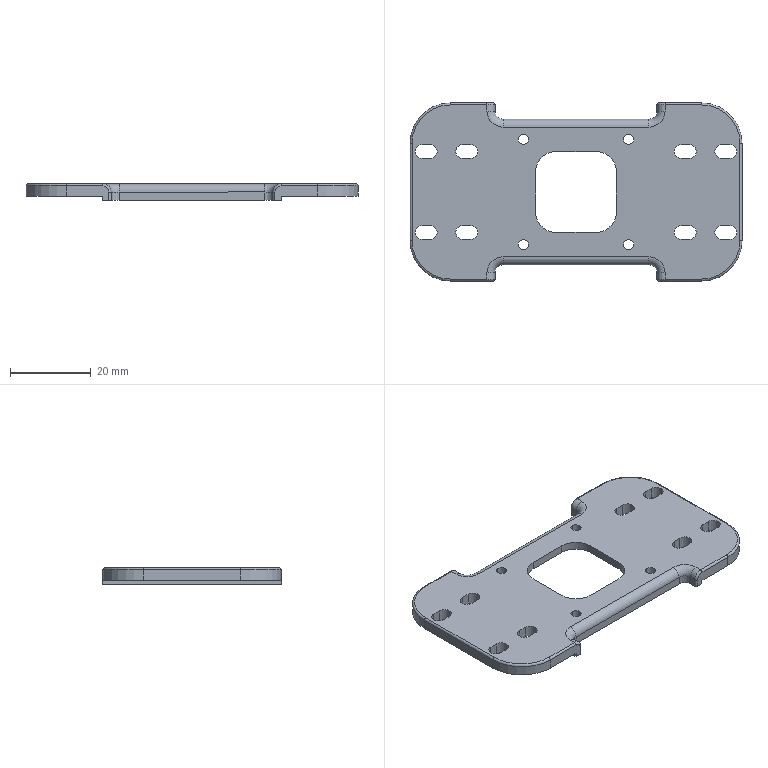NC program | NX | posted with a generic post | part box 82 x 44 x 4 mm
Lines 5498 to 6362 of 6362:
(ZLEVEL_PROFILE_COPY , TOOL : D10JING)
N10934 T14 M6
N10936 G54
N10938 G17 G0 G90 X-47.916 Y-13.684 S9500 M3
N10940 G43 Z30. H14
N10942 Z-2.525
N10944 G94 G1 Z-3.525 F1000.
N10946 X-46.5 Y-12.866
N10948 G3 X-46. Y-12. R1.
N10950 G1 Y12. F1200.
N10952 G2 X-31. Y27. R15.
N10954 G1 X-20.5
N10956 G2 X-15.208 Y23. R5.5
N10958 G1 X15.208
N10960 G2 X20.5 Y27. R5.5
N10962 G1 X31.
N10964 G2 X46. Y12. R15.
N10966 G1 Y-12.
N10968 G2 X31. Y-27. R15.
N10970 G1 X20.5
N10972 G2 X15.209 Y-23. R5.5
N10974 G1 X-15.208
N10976 G2 X-20.5 Y-27. R5.5
N10978 G1 X-31.
N10980 G2 X-46. Y-12. R15.
N10982 G1 Y12. Z-3.536
N10984 X-45.99 Y12.535
N10986 X-45.962 Y13.07
N10988 X-45.914 Y13.603 Z-3.537
N10990 X-45.847 Y14.135
N10992 X-45.762 Y14.663
N10994 X-45.657 Y15.188
N10996 X-45.534 Y15.71 Z-3.538
N10998 X-45.392 Y16.226
N11000 X-45.232 Y16.737
N11002 X-45.054 Y17.242
N11004 X-44.858 Y17.74 Z-3.539
N11006 X-44.644 Y18.231
N11008 X-44.413 Y18.714
N11010 X-44.165 Y19.189
N11012 X-43.9 Y19.654 Z-3.54
N11014 X-43.619 Y20.11
N11016 X-43.321 Y20.555
N11018 X-43.008 Y20.989
N11020 X-42.68 Y21.412 Z-3.541
N11022 X-42.336 Y21.823
N11024 X-41.978 Y22.221
N11026 X-41.607 Y22.607
N11028 X-41.221 Y22.978 Z-3.542
N11030 X-40.823 Y23.336
N11032 X-40.412 Y23.68
N11034 X-39.989 Y24.008
N11036 X-39.555 Y24.321 Z-3.543
N11038 X-39.11 Y24.619
N11040 X-38.654 Y24.9
N11042 X-38.189 Y25.165
N11044 X-37.714 Y25.413 Z-3.544
N11046 X-37.231 Y25.644
N11048 X-36.74 Y25.858
N11050 X-36.242 Y26.054
N11052 X-35.737 Y26.232 Z-3.545
N11054 X-35.226 Y26.392
N11056 X-34.71 Y26.534
N11058 X-34.188 Y26.657
N11060 X-33.663 Y26.762 Z-3.546
N11062 X-33.135 Y26.847
N11064 X-32.603 Y26.914
N11066 X-32.07 Y26.962
N11068 X-31.535 Y26.99
N11070 X-31. Y27. Z-3.547
N11072 X-20.5 Z-3.552
N11074 X-20.177 Y26.99
N11076 X-19.854 Y26.962
N11078 X-19.534 Y26.915
N11080 X-19.217 Y26.848
N11082 X-18.905 Y26.764
N11084 X-18.598 Y26.661
N11086 X-18.298 Y26.54 Z-3.553
N11088 X-18.005 Y26.402
N11090 X-17.721 Y26.247
N11092 X-17.447 Y26.075
N11094 X-17.183 Y25.887
N11096 X-16.931 Y25.685
N11098 X-16.691 Y25.468
N11100 X-16.464 Y25.237 Z-3.554
N11102 X-16.252 Y24.993
N11104 X-16.054 Y24.737
N11106 X-15.871 Y24.47
N11108 X-15.704 Y24.193
N11110 X-15.554 Y23.906
N11112 X-15.421 Y23.611
N11114 X-15.307 Y23.312 Z-3.555
N11116 X-15.208 Y23.
N11118 X15.208 Z-3.569
N11120 X15.307 Y23.312
N11122 X15.421 Y23.611
N11124 X15.554 Y23.906
N11126 X15.704 Y24.193
N11128 X15.871 Y24.47
N11130 X16.054 Y24.737 Z-3.57
N11132 X16.252 Y24.993
N11134 X16.464 Y25.237
N11136 X16.691 Y25.468
N11138 X16.931 Y25.685
N11140 X17.183 Y25.887
N11142 X17.447 Y26.075
N11144 X17.721 Y26.247 Z-3.571
N11146 X18.005 Y26.402
N11148 X18.298 Y26.54
N11150 X18.598 Y26.661
N11152 X18.905 Y26.764
N11154 X19.217 Y26.848
N11156 X19.534 Y26.915
N11158 X19.854 Y26.962 Z-3.572
N11160 X20.177 Y26.99
N11162 X20.5 Y27.
N11164 X31. Z-3.577
N11166 X31.535 Y26.99
N11168 X32.07 Y26.962
N11170 X32.603 Y26.914
N11172 X33.135 Y26.847 Z-3.578
N11174 X33.663 Y26.762
N11176 X34.188 Y26.657
N11178 X34.71 Y26.534
N11180 X35.226 Y26.392 Z-3.579
N11182 X35.737 Y26.232
N11184 X36.242 Y26.054
N11186 X36.74 Y25.858
N11188 X37.231 Y25.644 Z-3.58
N11190 X37.714 Y25.413
N11192 X38.189 Y25.165
N11194 X38.654 Y24.9
N11196 X39.11 Y24.619 Z-3.581
N11198 X39.555 Y24.321
N11200 X39.989 Y24.008
N11202 X40.412 Y23.68
N11204 X40.823 Y23.336 Z-3.582
N11206 X41.221 Y22.978
N11208 X41.607 Y22.607
N11210 X41.978 Y22.221
N11212 X42.336 Y21.823 Z-3.583
N11214 X42.68 Y21.412
N11216 X43.008 Y20.989
N11218 X43.321 Y20.555
N11220 X43.619 Y20.11 Z-3.584
N11222 X43.9 Y19.654
N11224 X44.165 Y19.189
N11226 X44.413 Y18.714
N11228 X44.644 Y18.231 Z-3.585
N11230 X44.858 Y17.74
N11232 X45.054 Y17.242
N11234 X45.232 Y16.737
N11236 X45.392 Y16.226 Z-3.586
N11238 X45.534 Y15.71
N11240 X45.657 Y15.188
N11242 X45.762 Y14.663
N11244 X45.847 Y14.135 Z-3.587
N11246 X45.914 Y13.603
N11248 X45.962 Y13.07
N11250 X45.99 Y12.535
N11252 X46. Y12. Z-3.588
N11254 Y-12. Z-3.598
N11256 X45.99 Y-12.535 Z-3.599
N11258 X45.962 Y-13.07
N11260 X45.914 Y-13.603
N11262 X45.847 Y-14.135
N11264 X45.762 Y-14.663 Z-3.6
N11266 X45.657 Y-15.188
N11268 X45.534 Y-15.71
N11270 X45.392 Y-16.226
N11272 X45.232 Y-16.737 Z-3.601
N11274 X45.054 Y-17.242
N11276 X44.858 Y-17.74
N11278 X44.644 Y-18.231
N11280 X44.413 Y-18.714 Z-3.602
N11282 X44.165 Y-19.189
N11284 X43.9 Y-19.654
N11286 X43.619 Y-20.11
N11288 X43.321 Y-20.555 Z-3.603
N11290 X43.008 Y-20.989
N11292 X42.68 Y-21.412
N11294 X42.336 Y-21.823
N11296 X41.978 Y-22.221 Z-3.604
N11298 X41.607 Y-22.607
N11300 X41.221 Y-22.978
N11302 X40.823 Y-23.336
N11304 X40.412 Y-23.68 Z-3.605
N11306 X39.989 Y-24.008
N11308 X39.555 Y-24.321
N11310 X39.11 Y-24.619
N11312 X38.654 Y-24.9 Z-3.606
N11314 X38.189 Y-25.165
N11316 X37.714 Y-25.413
N11318 X37.231 Y-25.644
N11320 X36.74 Y-25.858 Z-3.607
N11322 X36.242 Y-26.054
N11324 X35.737 Y-26.232
N11326 X35.226 Y-26.392
N11328 X34.71 Y-26.534 Z-3.608
N11330 X34.188 Y-26.657
N11332 X33.663 Y-26.762
N11334 X33.135 Y-26.847
N11336 X32.603 Y-26.914 Z-3.609
N11338 X32.07 Y-26.962
N11340 X31.535 Y-26.99
N11342 X31. Y-27.
N11344 X20.5 Z-3.614
N11346 X20.177 Y-26.99
N11348 X19.854 Y-26.962
N11350 X19.534 Y-26.915
N11352 X19.217 Y-26.848 Z-3.615
N11354 X18.905 Y-26.764
N11356 X18.598 Y-26.661
N11358 X18.298 Y-26.54
N11360 X18.005 Y-26.402
N11362 X17.721 Y-26.247
N11364 X17.447 Y-26.075 Z-3.616
N11366 X17.183 Y-25.887
N11368 X16.931 Y-25.685
N11370 X16.691 Y-25.468
N11372 X16.464 Y-25.237
N11374 X16.252 Y-24.993
N11376 X16.054 Y-24.737
N11378 X15.871 Y-24.47 Z-3.617
N11380 X15.704 Y-24.193
N11382 X15.554 Y-23.906
N11384 X15.421 Y-23.611
N11386 X15.307 Y-23.312
N11388 X15.209 Y-23.
N11390 X-15.208 Z-3.631
N11392 X-15.307 Y-23.312
N11394 X-15.421 Y-23.611
N11396 X-15.554 Y-23.906 Z-3.632
N11398 X-15.704 Y-24.193
N11400 X-15.871 Y-24.47
N11402 X-16.054 Y-24.737
N11404 X-16.252 Y-24.993
N11406 X-16.464 Y-25.237
N11408 X-16.691 Y-25.468 Z-3.633
N11410 X-16.931 Y-25.685
N11412 X-17.183 Y-25.887
N11414 X-17.447 Y-26.075
N11416 X-17.721 Y-26.247
N11418 X-18.005 Y-26.402
N11420 X-18.298 Y-26.54
N11422 X-18.598 Y-26.661 Z-3.634
N11424 X-18.905 Y-26.764
N11426 X-19.217 Y-26.848
N11428 X-19.534 Y-26.915
N11430 X-19.854 Y-26.962
N11432 X-20.177 Y-26.99
N11434 X-20.5 Y-27.
N11436 X-31. Z-3.639
N11438 X-31.535 Y-26.99
N11440 X-32.07 Y-26.962 Z-3.64
N11442 X-32.603 Y-26.914
N11444 X-33.135 Y-26.847
N11446 X-33.663 Y-26.762
N11448 X-34.188 Y-26.657 Z-3.641
N11450 X-34.71 Y-26.534
N11452 X-35.226 Y-26.392
N11454 X-35.737 Y-26.232
N11456 X-36.242 Y-26.054 Z-3.642
N11458 X-36.74 Y-25.858
N11460 X-37.231 Y-25.644
N11462 X-37.714 Y-25.413
N11464 X-38.189 Y-25.165 Z-3.643
N11466 X-38.654 Y-24.9
N11468 X-39.11 Y-24.619
N11470 X-39.555 Y-24.321
N11472 X-39.989 Y-24.008 Z-3.644
N11474 X-40.412 Y-23.68
N11476 X-40.823 Y-23.336
N11478 X-41.221 Y-22.978
N11480 X-41.607 Y-22.607 Z-3.645
N11482 X-41.978 Y-22.221
N11484 X-42.336 Y-21.823
N11486 X-42.68 Y-21.412
N11488 X-43.008 Y-20.989 Z-3.646
N11490 X-43.321 Y-20.555
N11492 X-43.619 Y-20.11
N11494 X-43.9 Y-19.654
N11496 X-44.165 Y-19.189 Z-3.647
N11498 X-44.413 Y-18.714
N11500 X-44.644 Y-18.231
N11502 X-44.858 Y-17.74
N11504 X-45.054 Y-17.242 Z-3.648
N11506 X-45.232 Y-16.737
N11508 X-45.392 Y-16.226
N11510 X-45.534 Y-15.71
N11512 X-45.657 Y-15.188 Z-3.649
N11514 X-45.762 Y-14.663
N11516 X-45.847 Y-14.135
N11518 X-45.914 Y-13.603
N11520 X-45.962 Y-13.07 Z-3.65
N11522 X-45.99 Y-12.535
N11524 X-46. Y-12.
N11526 Y12. Z-3.661
N11528 X-45.99 Y12.535
N11530 X-45.962 Y13.07
N11532 X-45.914 Y13.603 Z-3.662
N11534 X-45.847 Y14.135
N11536 X-45.762 Y14.663
N11538 X-45.657 Y15.188
N11540 X-45.534 Y15.71 Z-3.663
N11542 X-45.392 Y16.226
N11544 X-45.232 Y16.737
N11546 X-45.054 Y17.242
N11548 X-44.858 Y17.74 Z-3.664
N11550 X-44.644 Y18.231
N11552 X-44.413 Y18.714
N11554 X-44.165 Y19.189
N11556 X-43.9 Y19.654 Z-3.665
N11558 X-43.619 Y20.11
N11560 X-43.321 Y20.555
N11562 X-43.008 Y20.989
N11564 X-42.68 Y21.412 Z-3.666
N11566 X-42.336 Y21.823
N11568 X-41.978 Y22.221
N11570 X-41.607 Y22.607
N11572 X-41.221 Y22.978 Z-3.667
N11574 X-40.823 Y23.336
N11576 X-40.412 Y23.68
N11578 X-39.989 Y24.008
N11580 X-39.555 Y24.321 Z-3.668
N11582 X-39.11 Y24.619
N11584 X-38.654 Y24.9
N11586 X-38.189 Y25.165
N11588 X-37.714 Y25.413 Z-3.669
N11590 X-37.231 Y25.644
N11592 X-36.74 Y25.858
N11594 X-36.242 Y26.054
N11596 X-35.737 Y26.232 Z-3.67
N11598 X-35.226 Y26.392
N11600 X-34.71 Y26.534
N11602 X-34.188 Y26.657
N11604 X-33.663 Y26.762 Z-3.671
N11606 X-33.135 Y26.847
N11608 X-32.603 Y26.914
N11610 X-32.07 Y26.962
N11612 X-31.535 Y26.99
N11614 X-31. Y27. Z-3.672
N11616 X-20.5 Z-3.677
N11618 X-20.177 Y26.99
N11620 X-19.854 Y26.962
N11622 X-19.534 Y26.915
N11624 X-19.217 Y26.848
N11626 X-18.905 Y26.764
N11628 X-18.598 Y26.661
N11630 X-18.298 Y26.54 Z-3.678
N11632 X-18.005 Y26.402
N11634 X-17.721 Y26.247
N11636 X-17.447 Y26.075
N11638 X-17.183 Y25.887
N11640 X-16.931 Y25.685
N11642 X-16.691 Y25.468
N11644 X-16.464 Y25.237 Z-3.679
N11646 X-16.252 Y24.993
N11648 X-16.054 Y24.737
N11650 X-15.871 Y24.47
N11652 X-15.704 Y24.193
N11654 X-15.554 Y23.906
N11656 X-15.421 Y23.611
N11658 X-15.307 Y23.312 Z-3.68
N11660 X-15.208 Y23.
N11662 X15.208 Z-3.694
N11664 X15.307 Y23.312
N11666 X15.421 Y23.611
N11668 X15.554 Y23.906
N11670 X15.704 Y24.193
N11672 X15.871 Y24.47
N11674 X16.054 Y24.737 Z-3.695
N11676 X16.252 Y24.993
N11678 X16.464 Y25.237
N11680 X16.691 Y25.468
N11682 X16.931 Y25.685
N11684 X17.183 Y25.887
N11686 X17.447 Y26.075
N11688 X17.721 Y26.247 Z-3.696
N11690 X18.005 Y26.402
N11692 X18.298 Y26.54
N11694 X18.598 Y26.661
N11696 X18.905 Y26.764
N11698 X19.217 Y26.848
N11700 X19.534 Y26.915
N11702 X19.854 Y26.962 Z-3.697
N11704 X20.177 Y26.99
N11706 X20.5 Y27.
N11708 X31. Z-3.702
N11710 X31.535 Y26.99
N11712 X32.07 Y26.962
N11714 X32.603 Y26.914
N11716 X33.135 Y26.847 Z-3.703
N11718 X33.663 Y26.762
N11720 X34.188 Y26.657
N11722 X34.71 Y26.534
N11724 X35.226 Y26.392 Z-3.704
N11726 X35.737 Y26.232
N11728 X36.242 Y26.054
N11730 X36.74 Y25.858
N11732 X37.231 Y25.644 Z-3.705
N11734 X37.714 Y25.413
N11736 X38.189 Y25.165
N11738 X38.654 Y24.9
N11740 X39.11 Y24.619 Z-3.706
N11742 X39.555 Y24.321
N11744 X39.989 Y24.008
N11746 X40.412 Y23.68
N11748 X40.823 Y23.336 Z-3.707
N11750 X41.221 Y22.978
N11752 X41.607 Y22.607
N11754 X41.978 Y22.221
N11756 X42.336 Y21.823 Z-3.708
N11758 X42.68 Y21.412
N11760 X43.008 Y20.989
N11762 X43.321 Y20.555
N11764 X43.619 Y20.11 Z-3.709
N11766 X43.9 Y19.654
N11768 X44.165 Y19.189
N11770 X44.413 Y18.714
N11772 X44.644 Y18.231 Z-3.71
N11774 X44.858 Y17.74
N11776 X45.054 Y17.242
N11778 X45.232 Y16.737
N11780 X45.392 Y16.226 Z-3.711
N11782 X45.534 Y15.71
N11784 X45.657 Y15.188
N11786 X45.762 Y14.663
N11788 X45.847 Y14.135 Z-3.712
N11790 X45.914 Y13.603
N11792 X45.962 Y13.07
N11794 X45.99 Y12.535
N11796 X46. Y12. Z-3.713
N11798 Y-12. Z-3.723
N11800 X45.99 Y-12.535 Z-3.724
N11802 X45.962 Y-13.07
N11804 X45.914 Y-13.603
N11806 X45.847 Y-14.135
N11808 X45.762 Y-14.663 Z-3.725
N11810 X45.657 Y-15.188
N11812 X45.534 Y-15.71
N11814 X45.392 Y-16.226
N11816 X45.232 Y-16.737 Z-3.726
N11818 X45.054 Y-17.242
N11820 X44.858 Y-17.74
N11822 X44.644 Y-18.231
N11824 X44.413 Y-18.714 Z-3.727
N11826 X44.165 Y-19.189
N11828 X43.9 Y-19.654
N11830 X43.619 Y-20.11
N11832 X43.321 Y-20.555 Z-3.728
N11834 X43.008 Y-20.989
N11836 X42.68 Y-21.412
N11838 X42.336 Y-21.823
N11840 X41.978 Y-22.221 Z-3.729
N11842 X41.607 Y-22.607
N11844 X41.221 Y-22.978
N11846 X40.823 Y-23.336
N11848 X40.412 Y-23.68 Z-3.73
N11850 X39.989 Y-24.008
N11852 X39.555 Y-24.321
N11854 X39.11 Y-24.619
N11856 X38.654 Y-24.9 Z-3.731
N11858 X38.189 Y-25.165
N11860 X37.714 Y-25.413
N11862 X37.231 Y-25.644
N11864 X36.74 Y-25.858 Z-3.732
N11866 X36.242 Y-26.054
N11868 X35.737 Y-26.232
N11870 X35.226 Y-26.392
N11872 X34.71 Y-26.534 Z-3.733
N11874 X34.188 Y-26.657
N11876 X33.663 Y-26.762
N11878 X33.135 Y-26.847
N11880 X32.603 Y-26.914 Z-3.734
N11882 X32.07 Y-26.962
N11884 X31.535 Y-26.99
N11886 X31. Y-27.
N11888 X20.5 Z-3.739
N11890 X20.177 Y-26.99
N11892 X19.854 Y-26.962
N11894 X19.534 Y-26.915
N11896 X19.217 Y-26.848 Z-3.74
N11898 X18.905 Y-26.764
N11900 X18.598 Y-26.661
N11902 X18.298 Y-26.54
N11904 X18.005 Y-26.402
N11906 X17.721 Y-26.247
N11908 X17.447 Y-26.075 Z-3.741
N11910 X17.183 Y-25.887
N11912 X16.931 Y-25.685
N11914 X16.691 Y-25.468
N11916 X16.464 Y-25.237
N11918 X16.252 Y-24.993
N11920 X16.054 Y-24.737
N11922 X15.871 Y-24.47 Z-3.742
N11924 X15.704 Y-24.193
N11926 X15.554 Y-23.906
N11928 X15.421 Y-23.611
N11930 X15.307 Y-23.312
N11932 X15.209 Y-23.
N11934 X-15.208 Z-3.756
N11936 X-15.307 Y-23.312
N11938 X-15.421 Y-23.611
N11940 X-15.554 Y-23.906 Z-3.757
N11942 X-15.704 Y-24.193
N11944 X-15.871 Y-24.47
N11946 X-16.054 Y-24.737
N11948 X-16.252 Y-24.993
N11950 X-16.464 Y-25.237
N11952 X-16.691 Y-25.468 Z-3.758
N11954 X-16.931 Y-25.685
N11956 X-17.183 Y-25.887
N11958 X-17.447 Y-26.075
N11960 X-17.721 Y-26.247
N11962 X-18.005 Y-26.402
N11964 X-18.298 Y-26.54
N11966 X-18.598 Y-26.661 Z-3.759
N11968 X-18.905 Y-26.764
N11970 X-19.217 Y-26.848
N11972 X-19.534 Y-26.915
N11974 X-19.854 Y-26.962
N11976 X-20.177 Y-26.99
N11978 X-20.5 Y-27.
N11980 X-31. Z-3.764
N11982 X-31.535 Y-26.99
N11984 X-32.07 Y-26.962 Z-3.765
N11986 X-32.603 Y-26.914
N11988 X-33.135 Y-26.847
N11990 X-33.663 Y-26.762
N11992 X-34.188 Y-26.657 Z-3.766
N11994 X-34.71 Y-26.534
N11996 X-35.226 Y-26.392
N11998 X-35.737 Y-26.232
N12000 X-36.242 Y-26.054 Z-3.767
N12002 X-36.74 Y-25.858
N12004 X-37.231 Y-25.644
N12006 X-37.714 Y-25.413
N12008 X-38.189 Y-25.165 Z-3.768
N12010 X-38.654 Y-24.9
N12012 X-39.11 Y-24.619
N12014 X-39.555 Y-24.321
N12016 X-39.989 Y-24.008 Z-3.769
N12018 X-40.412 Y-23.68
N12020 X-40.823 Y-23.336
N12022 X-41.221 Y-22.978
N12024 X-41.607 Y-22.607 Z-3.77
N12026 X-41.978 Y-22.221
N12028 X-42.336 Y-21.823
N12030 X-42.68 Y-21.412
N12032 X-43.008 Y-20.989 Z-3.771
N12034 X-43.321 Y-20.555
N12036 X-43.619 Y-20.11
N12038 X-43.9 Y-19.654
N12040 X-44.165 Y-19.189 Z-3.772
N12042 X-44.413 Y-18.714
N12044 X-44.644 Y-18.231
N12046 X-44.858 Y-17.74
N12048 X-45.054 Y-17.242 Z-3.773
N12050 X-45.232 Y-16.737
N12052 X-45.392 Y-16.226
N12054 X-45.534 Y-15.71
N12056 X-45.657 Y-15.188 Z-3.774
N12058 X-45.762 Y-14.663
N12060 X-45.847 Y-14.135
N12062 X-45.914 Y-13.603
N12064 X-45.962 Y-13.07 Z-3.775
N12066 X-45.99 Y-12.535
N12068 X-46. Y-12.
N12070 Y12. Z-3.786
N12072 X-45.99 Y12.535
N12074 X-45.962 Y13.07
N12076 X-45.914 Y13.603 Z-3.787
N12078 X-45.847 Y14.135
N12080 X-45.762 Y14.663
N12082 X-45.657 Y15.188
N12084 X-45.534 Y15.71 Z-3.788
N12086 X-45.392 Y16.226
N12088 X-45.232 Y16.737
N12090 X-45.054 Y17.242
N12092 X-44.858 Y17.74 Z-3.789
N12094 X-44.644 Y18.231
N12096 X-44.413 Y18.714
N12098 X-44.165 Y19.189
N12100 X-43.9 Y19.654 Z-3.79
N12102 X-43.619 Y20.11
N12104 X-43.321 Y20.555
N12106 X-43.008 Y20.989
N12108 X-42.68 Y21.412 Z-3.791
N12110 X-42.336 Y21.823
N12112 X-41.978 Y22.221
N12114 X-41.607 Y22.607
N12116 X-41.221 Y22.978 Z-3.792
N12118 X-40.823 Y23.336
N12120 X-40.412 Y23.68
N12122 X-39.989 Y24.008
N12124 X-39.555 Y24.321 Z-3.793
N12126 X-39.11 Y24.619
N12128 X-38.654 Y24.9
N12130 X-38.189 Y25.165
N12132 X-37.714 Y25.413 Z-3.794
N12134 X-37.231 Y25.644
N12136 X-36.74 Y25.858
N12138 X-36.242 Y26.054
N12140 X-35.737 Y26.232 Z-3.795
N12142 X-35.226 Y26.392
N12144 X-34.71 Y26.534
N12146 X-34.188 Y26.657
N12148 X-33.663 Y26.762 Z-3.796
N12150 X-33.135 Y26.847
N12152 X-32.603 Y26.914
N12154 X-32.07 Y26.962
N12156 X-31.535 Y26.99
N12158 X-31. Y27. Z-3.797
N12160 X-20.5 Z-3.802
N12162 X-20.177 Y26.99
N12164 X-19.854 Y26.962
N12166 X-19.534 Y26.915
N12168 X-19.217 Y26.848
N12170 X-18.905 Y26.764
N12172 X-18.598 Y26.661
N12174 X-18.298 Y26.54 Z-3.803
N12176 X-18.005 Y26.402
N12178 X-17.721 Y26.247
N12180 X-17.447 Y26.075
N12182 X-17.183 Y25.887
N12184 X-16.931 Y25.685
N12186 X-16.691 Y25.468
N12188 X-16.464 Y25.237 Z-3.804
N12190 X-16.252 Y24.993
N12192 X-16.054 Y24.737
N12194 X-15.871 Y24.47
N12196 X-15.704 Y24.193
N12198 X-15.554 Y23.906
N12200 X-15.421 Y23.611
N12202 X-15.307 Y23.312 Z-3.805
N12204 X-15.208 Y23.
N12206 X15.208 Z-3.819
N12208 X15.307 Y23.312
N12210 X15.421 Y23.611
N12212 X15.554 Y23.906
N12214 X15.704 Y24.193
N12216 X15.871 Y24.47
N12218 X16.054 Y24.737 Z-3.82
N12220 X16.252 Y24.993
N12222 X16.464 Y25.237
N12224 X16.691 Y25.468
N12226 X16.931 Y25.685
N12228 X17.183 Y25.887
N12230 X17.447 Y26.075
N12232 X17.721 Y26.247 Z-3.821
N12234 X18.005 Y26.402
N12236 X18.298 Y26.54
N12238 X18.598 Y26.661
N12240 X18.905 Y26.764
N12242 X19.217 Y26.848
N12244 X19.534 Y26.915
N12246 X19.854 Y26.962 Z-3.822
N12248 X20.177 Y26.99
N12250 X20.5 Y27.
N12252 X31. Z-3.827
N12254 X31.535 Y26.99
N12256 X32.07 Y26.962
N12258 X32.603 Y26.914
N12260 X33.135 Y26.847 Z-3.828
N12262 X33.663 Y26.762
N12264 X34.188 Y26.657
N12266 X34.71 Y26.534
N12268 X35.226 Y26.392 Z-3.829
N12270 X35.737 Y26.232
N12272 X36.242 Y26.054
N12274 X36.74 Y25.858
N12276 X37.231 Y25.644 Z-3.83
N12278 X37.714 Y25.413
N12280 X38.189 Y25.165
N12282 X38.654 Y24.9
N12284 X39.11 Y24.619 Z-3.831
N12286 X39.555 Y24.321
N12288 X39.989 Y24.008
N12290 X40.412 Y23.68
N12292 X40.823 Y23.336 Z-3.832
N12294 X41.221 Y22.978
N12296 X41.607 Y22.607
N12298 X41.978 Y22.221
N12300 X42.336 Y21.823 Z-3.833
N12302 X42.68 Y21.412
N12304 X43.008 Y20.989
N12306 X43.321 Y20.555
N12308 X43.619 Y20.11 Z-3.834
N12310 X43.9 Y19.654
N12312 X44.165 Y19.189
N12314 X44.413 Y18.714
N12316 X44.644 Y18.231 Z-3.835
N12318 X44.858 Y17.74
N12320 X45.054 Y17.242
N12322 X45.232 Y16.737
N12324 X45.392 Y16.226 Z-3.836
N12326 X45.534 Y15.71
N12328 X45.657 Y15.188
N12330 X45.762 Y14.663
N12332 X45.847 Y14.135 Z-3.837
N12334 X45.914 Y13.603
N12336 X45.962 Y13.07
N12338 X45.99 Y12.535
N12340 X46. Y12. Z-3.838
N12342 Y-12. Z-3.848
N12344 X45.99 Y-12.535 Z-3.849
N12346 X45.962 Y-13.07
N12348 X45.914 Y-13.603
N12350 X45.847 Y-14.135
N12352 X45.762 Y-14.663 Z-3.85
N12354 X45.657 Y-15.188
N12356 X45.534 Y-15.71
N12358 X45.392 Y-16.226
N12360 X45.232 Y-16.737 Z-3.851
N12362 X45.054 Y-17.242
N12364 X44.858 Y-17.74
N12366 X44.644 Y-18.231
N12368 X44.413 Y-18.714 Z-3.852
N12370 X44.165 Y-19.189
N12372 X43.9 Y-19.654
N12374 X43.619 Y-20.11
N12376 X43.321 Y-20.555 Z-3.853
N12378 X43.008 Y-20.989
N12380 X42.68 Y-21.412
N12382 X42.336 Y-21.823
N12384 X41.978 Y-22.221 Z-3.854
N12386 X41.607 Y-22.607
N12388 X41.221 Y-22.978
N12390 X40.823 Y-23.336
N12392 X40.412 Y-23.68 Z-3.855
N12394 X39.989 Y-24.008
N12396 X39.555 Y-24.321
N12398 X39.11 Y-24.619
N12400 X38.654 Y-24.9 Z-3.856
N12402 X38.189 Y-25.165
N12404 X37.714 Y-25.413
N12406 X37.231 Y-25.644
N12408 X36.74 Y-25.858 Z-3.857
N12410 X36.242 Y-26.054
N12412 X35.737 Y-26.232
N12414 X35.226 Y-26.392
N12416 X34.71 Y-26.534 Z-3.858
N12418 X34.188 Y-26.657
N12420 X33.663 Y-26.762
N12422 X33.135 Y-26.847
N12424 X32.603 Y-26.914 Z-3.859
N12426 X32.07 Y-26.962
N12428 X31.535 Y-26.99
N12430 X31. Y-27.
N12432 X20.5 Z-3.864
N12434 X20.177 Y-26.99
N12436 X19.854 Y-26.962
N12438 X19.534 Y-26.915
N12440 X19.217 Y-26.848 Z-3.865
N12442 X18.905 Y-26.764
N12444 X18.598 Y-26.661
N12446 X18.298 Y-26.54
N12448 X18.005 Y-26.402
N12450 X17.721 Y-26.247
N12452 X17.447 Y-26.075 Z-3.866
N12454 X17.183 Y-25.887
N12456 X16.931 Y-25.685
N12458 X16.691 Y-25.468
N12460 X16.464 Y-25.237
N12462 X16.252 Y-24.993
N12464 X16.054 Y-24.737
N12466 X15.871 Y-24.47 Z-3.867
N12468 X15.704 Y-24.193
N12470 X15.554 Y-23.906
N12472 X15.421 Y-23.611
N12474 X15.307 Y-23.312
N12476 X15.209 Y-23.
N12478 X-15.208 Z-3.881
N12480 X-15.307 Y-23.312
N12482 X-15.421 Y-23.611
N12484 X-15.554 Y-23.906 Z-3.882
N12486 X-15.704 Y-24.193
N12488 X-15.871 Y-24.47
N12490 X-16.054 Y-24.737
N12492 X-16.252 Y-24.993
N12494 X-16.464 Y-25.237
N12496 X-16.691 Y-25.468 Z-3.883
N12498 X-16.931 Y-25.685
N12500 X-17.183 Y-25.887
N12502 X-17.447 Y-26.075
N12504 X-17.721 Y-26.247
N12506 X-18.005 Y-26.402
N12508 X-18.298 Y-26.54
N12510 X-18.598 Y-26.661 Z-3.884
N12512 X-18.905 Y-26.764
N12514 X-19.217 Y-26.848
N12516 X-19.534 Y-26.915
N12518 X-19.854 Y-26.962
N12520 X-20.177 Y-26.99
N12522 X-20.5 Y-27.
N12524 X-31. Z-3.889
N12526 X-31.535 Y-26.99
N12528 X-32.07 Y-26.962 Z-3.89
N12530 X-32.603 Y-26.914
N12532 X-33.135 Y-26.847
N12534 X-33.663 Y-26.762
N12536 X-34.188 Y-26.657 Z-3.891
N12538 X-34.71 Y-26.534
N12540 X-35.226 Y-26.392
N12542 X-35.737 Y-26.232
N12544 X-36.242 Y-26.054 Z-3.892
N12546 X-36.74 Y-25.858
N12548 X-37.231 Y-25.644
N12550 X-37.714 Y-25.413
N12552 X-38.189 Y-25.165 Z-3.893
N12554 X-38.654 Y-24.9
N12556 X-39.11 Y-24.619
N12558 X-39.555 Y-24.321
N12560 X-39.989 Y-24.008 Z-3.894
N12562 X-40.412 Y-23.68
N12564 X-40.823 Y-23.336
N12566 X-41.221 Y-22.978
N12568 X-41.607 Y-22.607 Z-3.895
N12570 X-41.978 Y-22.221
N12572 X-42.336 Y-21.823
N12574 X-42.68 Y-21.412
N12576 X-43.008 Y-20.989 Z-3.896
N12578 X-43.321 Y-20.555
N12580 X-43.619 Y-20.11
N12582 X-43.9 Y-19.654
N12584 X-44.165 Y-19.189 Z-3.897
N12586 X-44.413 Y-18.714
N12588 X-44.644 Y-18.231
N12590 X-44.858 Y-17.74
N12592 X-45.054 Y-17.242 Z-3.898
N12594 X-45.232 Y-16.737
N12596 X-45.392 Y-16.226
N12598 X-45.534 Y-15.71
N12600 X-45.657 Y-15.188 Z-3.899
N12602 X-45.762 Y-14.663
N12604 X-45.847 Y-14.135
N12606 X-45.914 Y-13.603
N12608 X-45.962 Y-13.07 Z-3.9
N12610 X-45.99 Y-12.535
N12612 X-46. Y-12.
N12614 Y12.
N12616 G2 X-31. Y27. R15.
N12618 G1 X-20.5
N12620 G2 X-15.208 Y23. R5.5
N12622 G1 X15.208
N12624 G2 X20.5 Y27. R5.5
N12626 G1 X31.
N12628 G2 X46. Y12. R15.
N12630 G1 Y-12.
N12632 G2 X31. Y-27. R15.
N12634 G1 X20.5
N12636 G2 X15.209 Y-23. R5.5
N12638 G1 X-15.208
N12640 G2 X-20.5 Y-27. R5.5
N12642 G1 X-31.
N12644 G2 X-46. Y-12. R15.
N12646 G3 X-46.5 Y-11.134 R1.
N12648 G1 X-48. Y-10.268
N12650 Z-2.9
N12652 G0 Z30.
N12654 M5
N12656 M2